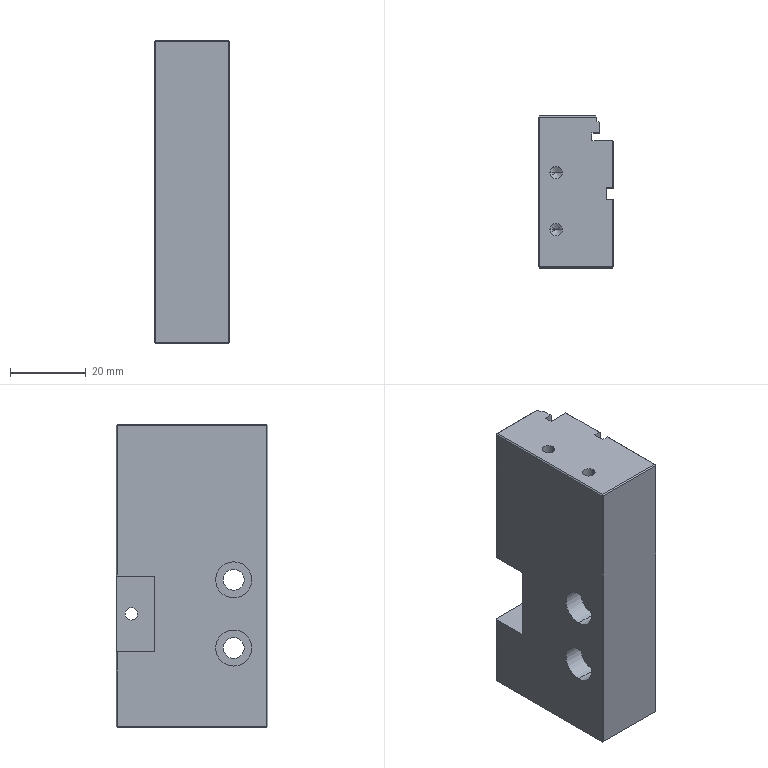Part | STEP file | Rivet push-in slide_Default | 1 solid | 68 faces | box 20 x 40 x 80 mm | volume 57141 mm3 | plane 46 | cylinder 16 | cone 6 | commonest cylinder face diameters 3.3 x6 5.5 x4 9.5 x4 4.2 x2